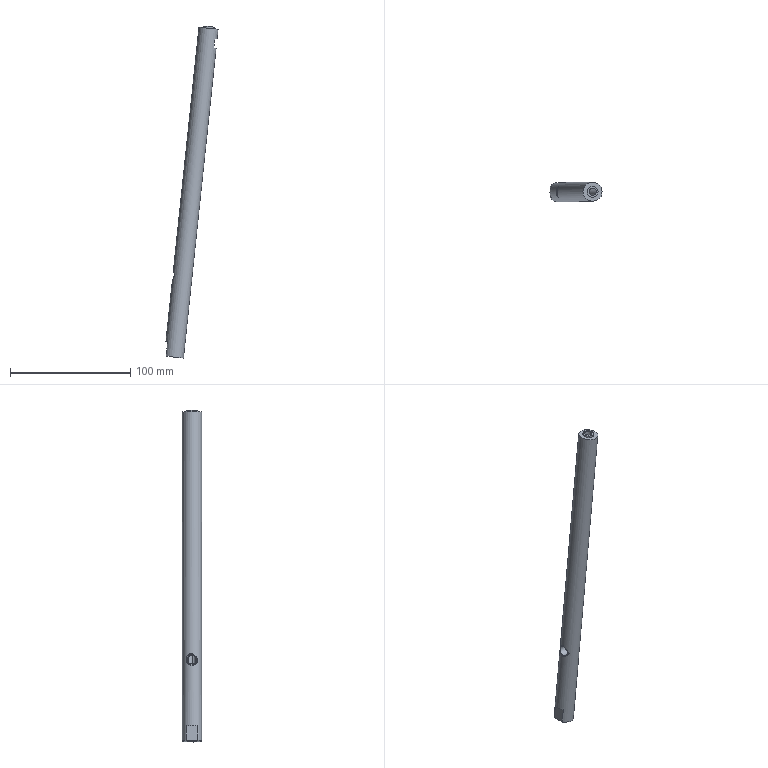Part | STEP file | P011002L001-001 | 1 solid | 88 faces | box 43.362 x 16 x 275.795 mm | volume 48038 mm3 | plane 40 | cone 19 | other 13 | cylinder 12 | spline 4 | commonest cylinder face diameters 6 x5 8 x2 16 x2 6.8 x1 7.973 x1 9 x1